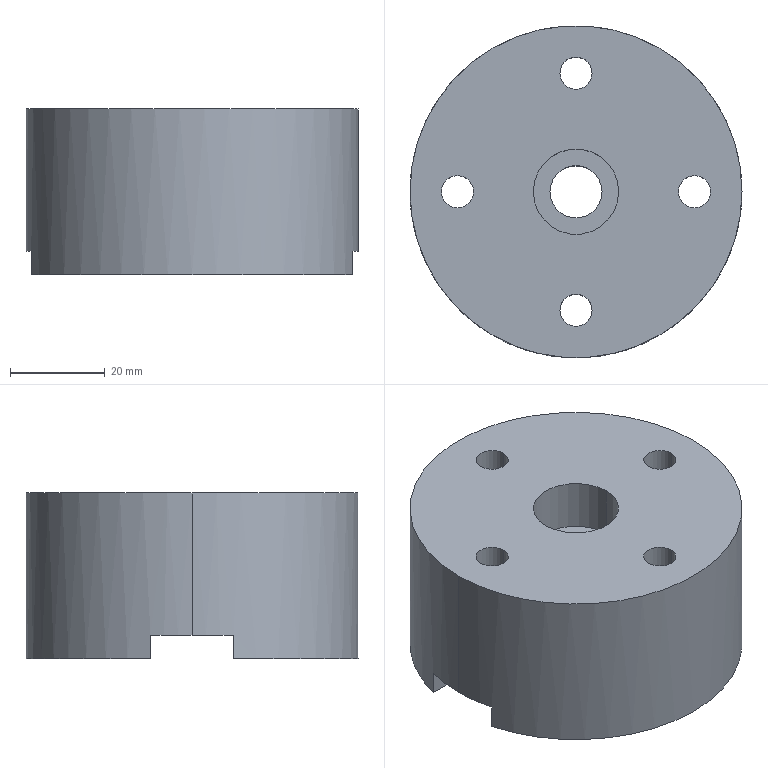Part | SolidWorks | features BaseBody 1 | 1 solid | 21 faces | box 70 x 70 x 35 mm | volume 119309 mm3 | cylinder 14 | plane 7 | commonest cylinder face diameters 6.8 x8 11 x2 18 x2 70 x2
STEP:
#1=CARTESIAN_POINT('',(-3.4,25.,35.));
#2=VERTEX_POINT('',#1);
#3=CARTESIAN_POINT('',(3.4,25.,35.));
#4=VERTEX_POINT('',#3);
#5=CARTESIAN_POINT('',(0.,25.,35.));
#6=DIRECTION('',(0.,0.,1.));
#7=DIRECTION('',(1.,0.,0.));
#8=AXIS2_PLACEMENT_3D('',#5,#6,#7);
#9=CIRCLE('',#8,3.4);
#10=EDGE_CURVE('',#2,#4,#9,.T.);
#11=ORIENTED_EDGE('',*,*,#10,.T.);
#12=CARTESIAN_POINT('',(3.4,25.,0.));
#13=VERTEX_POINT('',#12);
#14=CARTESIAN_POINT('',(3.4,25.,0.));
#15=DIRECTION('',(0.,0.,-1.));
#16=VECTOR('',#15,1000.);
#17=LINE('',#14,#16);
#18=EDGE_CURVE('',#4,#13,#17,.T.);
#19=ORIENTED_EDGE('',*,*,#18,.T.);
#20=CARTESIAN_POINT('',(-3.4,25.,0.));
#21=VERTEX_POINT('',#20);
#22=CARTESIAN_POINT('',(0.,25.,0.));
#23=DIRECTION('',(0.,0.,-1.));
#24=DIRECTION('',(-1.,0.,0.));
#25=AXIS2_PLACEMENT_3D('',#22,#23,#24);
#26=CIRCLE('',#25,3.4);
#27=EDGE_CURVE('',#13,#21,#26,.T.);
#28=ORIENTED_EDGE('',*,*,#27,.T.);
#29=CARTESIAN_POINT('',(-3.4,25.,0.));
#30=DIRECTION('',(0.,0.,-1.));
#31=VECTOR('',#30,1000.);
#32=LINE('',#29,#31);
#33=EDGE_CURVE('',#2,#21,#32,.T.);
#34=ORIENTED_EDGE('',*,*,#33,.F.);
#35=EDGE_LOOP('',(#11,#19,#28,#34));
#36=FACE_OUTER_BOUND('',#35,.T.);
#37=CARTESIAN_POINT('',(0.,25.,0.));
#38=DIRECTION('',(0.,0.,-1.));
#39=DIRECTION('',(-1.,0.,0.));
#40=AXIS2_PLACEMENT_3D('',#37,#38,#39);
#41=CYLINDRICAL_SURFACE('',#40,3.4);
#42=ADVANCED_FACE('',(#36),#41,.F.);
#43=CARTESIAN_POINT('',(21.6,0.,35.));
#44=VERTEX_POINT('',#43);
#45=CARTESIAN_POINT('',(28.4,0.,35.));
#46=VERTEX_POINT('',#45);
#47=CARTESIAN_POINT('',(25.,0.,35.));
#48=DIRECTION('',(0.,0.,1.));
#49=DIRECTION('',(1.,0.,0.));
#50=AXIS2_PLACEMENT_3D('',#47,#48,#49);
#51=CIRCLE('',#50,3.4);
#52=EDGE_CURVE('',#44,#46,#51,.T.);
#53=ORIENTED_EDGE('',*,*,#52,.T.);
#54=CARTESIAN_POINT('',(28.4,0.,5.));
#55=VERTEX_POINT('',#54);
#56=CARTESIAN_POINT('',(28.4,0.,0.));
#57=DIRECTION('',(0.,0.,-1.));
#58=VECTOR('',#57,1000.);
#59=LINE('',#56,#58);
#60=EDGE_CURVE('',#46,#55,#59,.T.);
#61=ORIENTED_EDGE('',*,*,#60,.T.);
#62=CARTESIAN_POINT('',(21.6,0.,5.));
#63=VERTEX_POINT('',#62);
#64=CARTESIAN_POINT('',(25.,0.,5.));
#65=DIRECTION('',(0.,0.,1.));
#66=DIRECTION('',(1.,0.,0.));
#67=AXIS2_PLACEMENT_3D('',#64,#65,#66);
#68=CIRCLE('',#67,3.4);
#69=EDGE_CURVE('',#63,#55,#68,.T.);
#70=ORIENTED_EDGE('',*,*,#69,.F.);
#71=CARTESIAN_POINT('',(21.6,0.,0.));
#72=DIRECTION('',(0.,0.,-1.));
#73=VECTOR('',#72,1000.);
#74=LINE('',#71,#73);
#75=EDGE_CURVE('',#44,#63,#74,.T.);
#76=ORIENTED_EDGE('',*,*,#75,.F.);
#77=EDGE_LOOP('',(#53,#61,#70,#76));
#78=FACE_OUTER_BOUND('',#77,.T.);
#79=CARTESIAN_POINT('',(25.,0.,0.));
#80=DIRECTION('',(0.,0.,-1.));
#81=DIRECTION('',(-1.,0.,0.));
#82=AXIS2_PLACEMENT_3D('',#79,#80,#81);
#83=CYLINDRICAL_SURFACE('',#82,3.4);
#84=ADVANCED_FACE('',(#78),#83,.F.);
#85=CARTESIAN_POINT('',(-28.4,0.,35.));
#86=VERTEX_POINT('',#85);
#87=CARTESIAN_POINT('',(-21.6,0.,35.));
#88=VERTEX_POINT('',#87);
#89=CARTESIAN_POINT('',(-25.,0.,35.));
#90=DIRECTION('',(0.,0.,1.));
#91=DIRECTION('',(1.,0.,0.));
#92=AXIS2_PLACEMENT_3D('',#89,#90,#91);
#93=CIRCLE('',#92,3.4);
#94=EDGE_CURVE('',#86,#88,#93,.T.);
#95=ORIENTED_EDGE('',*,*,#94,.T.);
#96=CARTESIAN_POINT('',(-21.6,0.,5.));
#97=VERTEX_POINT('',#96);
#98=CARTESIAN_POINT('',(-21.6,0.,0.));
#99=DIRECTION('',(0.,0.,-1.));
#100=VECTOR('',#99,1000.);
#101=LINE('',#98,#100);
#102=EDGE_CURVE('',#88,#97,#101,.T.);
#103=ORIENTED_EDGE('',*,*,#102,.T.);
#104=CARTESIAN_POINT('',(-28.4,0.,5.));
#105=VERTEX_POINT('',#104);
#106=CARTESIAN_POINT('',(-25.,0.,5.));
#107=DIRECTION('',(0.,0.,1.));
#108=DIRECTION('',(1.,0.,0.));
#109=AXIS2_PLACEMENT_3D('',#106,#107,#108);
#110=CIRCLE('',#109,3.4);
#111=EDGE_CURVE('',#105,#97,#110,.T.);
#112=ORIENTED_EDGE('',*,*,#111,.F.);
#113=CARTESIAN_POINT('',(-28.4,0.,0.));
#114=DIRECTION('',(0.,0.,-1.));
#115=VECTOR('',#114,1000.);
#116=LINE('',#113,#115);
#117=EDGE_CURVE('',#86,#105,#116,.T.);
#118=ORIENTED_EDGE('',*,*,#117,.F.);
#119=EDGE_LOOP('',(#95,#103,#112,#118));
#120=FACE_OUTER_BOUND('',#119,.T.);
#121=CARTESIAN_POINT('',(-25.,0.,0.));
#122=DIRECTION('',(0.,0.,-1.));
#123=DIRECTION('',(-1.,0.,0.));
#124=AXIS2_PLACEMENT_3D('',#121,#122,#123);
#125=CYLINDRICAL_SURFACE('',#124,3.4);
#126=ADVANCED_FACE('',(#120),#125,.F.);
#127=CARTESIAN_POINT('',(-3.4,-25.,35.));
#128=VERTEX_POINT('',#127);
#129=CARTESIAN_POINT('',(3.4,-25.,35.));
#130=VERTEX_POINT('',#129);
#131=CARTESIAN_POINT('',(0.,-25.,35.));
#132=DIRECTION('',(0.,0.,1.));
#133=DIRECTION('',(1.,0.,0.));
#134=AXIS2_PLACEMENT_3D('',#131,#132,#133);
#135=CIRCLE('',#134,3.4);
#136=EDGE_CURVE('',#128,#130,#135,.T.);
#137=ORIENTED_EDGE('',*,*,#136,.T.);
#138=CARTESIAN_POINT('',(3.4,-25.,0.));
#139=VERTEX_POINT('',#138);
#140=CARTESIAN_POINT('',(3.4,-25.,0.));
#141=DIRECTION('',(0.,0.,-1.));
#142=VECTOR('',#141,1000.);
#143=LINE('',#140,#142);
#144=EDGE_CURVE('',#130,#139,#143,.T.);
#145=ORIENTED_EDGE('',*,*,#144,.T.);
#146=CARTESIAN_POINT('',(-3.4,-25.,0.));
#147=VERTEX_POINT('',#146);
#148=CARTESIAN_POINT('',(0.,-25.,0.));
#149=DIRECTION('',(0.,0.,-1.));
#150=DIRECTION('',(-1.,0.,0.));
#151=AXIS2_PLACEMENT_3D('',#148,#149,#150);
#152=CIRCLE('',#151,3.4);
#153=EDGE_CURVE('',#139,#147,#152,.T.);
#154=ORIENTED_EDGE('',*,*,#153,.T.);
#155=CARTESIAN_POINT('',(-3.4,-25.,0.));
#156=DIRECTION('',(0.,0.,-1.));
#157=VECTOR('',#156,1000.);
#158=LINE('',#155,#157);
#159=EDGE_CURVE('',#128,#147,#158,.T.);
#160=ORIENTED_EDGE('',*,*,#159,.F.);
#161=EDGE_LOOP('',(#137,#145,#154,#160));
#162=FACE_OUTER_BOUND('',#161,.T.);
#163=CARTESIAN_POINT('',(0.,-25.,0.));
#164=DIRECTION('',(0.,0.,-1.));
#165=DIRECTION('',(-1.,0.,0.));
#166=AXIS2_PLACEMENT_3D('',#163,#164,#165);
#167=CYLINDRICAL_SURFACE('',#166,3.4);
#168=ADVANCED_FACE('',(#162),#167,.F.);
#169=CARTESIAN_POINT('',(-9.,0.,24.));
#170=VERTEX_POINT('',#169);
#171=CARTESIAN_POINT('',(9.,0.,24.));
#172=VERTEX_POINT('',#171);
#173=CARTESIAN_POINT('',(0.,0.,24.));
#174=DIRECTION('',(0.,0.,1.));
#175=DIRECTION('',(1.,0.,0.));
#176=AXIS2_PLACEMENT_3D('',#173,#174,#175);
#177=CIRCLE('',#176,9.);
#178=EDGE_CURVE('',#170,#172,#177,.T.);
#179=ORIENTED_EDGE('',*,*,#178,.F.);
#180=CARTESIAN_POINT('',(-9.,0.,35.));
#181=VERTEX_POINT('',#180);
#182=CARTESIAN_POINT('',(-9.,0.,35.));
#183=DIRECTION('',(0.,0.,1.));
#184=VECTOR('',#183,1000.);
#185=LINE('',#182,#184);
#186=EDGE_CURVE('',#170,#181,#185,.T.);
#187=ORIENTED_EDGE('',*,*,#186,.T.);
#188=CARTESIAN_POINT('',(9.,0.,35.));
#189=VERTEX_POINT('',#188);
#190=CARTESIAN_POINT('',(0.,0.,35.));
#191=DIRECTION('',(0.,0.,1.));
#192=DIRECTION('',(1.,0.,0.));
#193=AXIS2_PLACEMENT_3D('',#190,#191,#192);
#194=CIRCLE('',#193,9.);
#195=EDGE_CURVE('',#181,#189,#194,.T.);
#196=ORIENTED_EDGE('',*,*,#195,.T.);
#197=CARTESIAN_POINT('',(9.,0.,35.));
#198=DIRECTION('',(0.,0.,1.));
#199=VECTOR('',#198,1000.);
#200=LINE('',#197,#199);
#201=EDGE_CURVE('',#172,#189,#200,.T.);
#202=ORIENTED_EDGE('',*,*,#201,.F.);
#203=EDGE_LOOP('',(#179,#187,#196,#202));
#204=FACE_OUTER_BOUND('',#203,.T.);
#205=CARTESIAN_POINT('',(0.,0.,35.));
#206=DIRECTION('',(0.,0.,1.));
#207=DIRECTION('',(1.,0.,0.));
#208=AXIS2_PLACEMENT_3D('',#205,#206,#207);
#209=CYLINDRICAL_SURFACE('',#208,9.);
#210=ADVANCED_FACE('',(#204),#209,.F.);
#211=CARTESIAN_POINT('',(-5.5,0.,5.));
#212=VERTEX_POINT('',#211);
#213=CARTESIAN_POINT('',(5.5,0.,5.));
#214=VERTEX_POINT('',#213);
#215=CARTESIAN_POINT('',(0.,0.,5.));
#216=DIRECTION('',(0.,0.,1.));
#217=DIRECTION('',(1.,0.,0.));
#218=AXIS2_PLACEMENT_3D('',#215,#216,#217);
#219=CIRCLE('',#218,5.5);
#220=EDGE_CURVE('',#212,#214,#219,.T.);
#221=ORIENTED_EDGE('',*,*,#220,.F.);
#222=CARTESIAN_POINT('',(-5.5,0.,24.));
#223=VERTEX_POINT('',#222);
#224=CARTESIAN_POINT('',(-5.5,0.,35.));
#225=DIRECTION('',(0.,0.,1.));
#226=VECTOR('',#225,1000.);
#227=LINE('',#224,#226);
#228=EDGE_CURVE('',#212,#223,#227,.T.);
#229=ORIENTED_EDGE('',*,*,#228,.T.);
#230=CARTESIAN_POINT('',(5.5,0.,24.));
#231=VERTEX_POINT('',#230);
#232=CARTESIAN_POINT('',(0.,0.,24.));
#233=DIRECTION('',(0.,0.,1.));
#234=DIRECTION('',(1.,0.,0.));
#235=AXIS2_PLACEMENT_3D('',#232,#233,#234);
#236=CIRCLE('',#235,5.5);
#237=EDGE_CURVE('',#223,#231,#236,.T.);
#238=ORIENTED_EDGE('',*,*,#237,.T.);
#239=CARTESIAN_POINT('',(5.5,0.,35.));
#240=DIRECTION('',(0.,0.,1.));
#241=VECTOR('',#240,1000.);
#242=LINE('',#239,#241);
#243=EDGE_CURVE('',#214,#231,#242,.T.);
#244=ORIENTED_EDGE('',*,*,#243,.F.);
#245=EDGE_LOOP('',(#221,#229,#238,#244));
#246=FACE_OUTER_BOUND('',#245,.T.);
#247=CARTESIAN_POINT('',(0.,0.,35.));
#248=DIRECTION('',(0.,0.,1.));
#249=DIRECTION('',(1.,0.,0.));
#250=AXIS2_PLACEMENT_3D('',#247,#248,#249);
#251=CYLINDRICAL_SURFACE('',#250,5.5);
#252=ADVANCED_FACE('',(#246),#251,.F.);
#253=CARTESIAN_POINT('',(35.,0.,35.));
#254=VERTEX_POINT('',#253);
#255=CARTESIAN_POINT('',(-35.,0.,35.));
#256=VERTEX_POINT('',#255);
#257=CARTESIAN_POINT('',(0.,0.,35.));
#258=DIRECTION('',(0.,0.,1.));
#259=DIRECTION('',(1.,0.,0.));
#260=AXIS2_PLACEMENT_3D('',#257,#258,#259);
#261=CIRCLE('',#260,35.);
#262=EDGE_CURVE('',#254,#256,#261,.T.);
#263=ORIENTED_EDGE('',*,*,#262,.F.);
#264=CARTESIAN_POINT('',(35.,0.,5.));
#265=VERTEX_POINT('',#264);
#266=CARTESIAN_POINT('',(35.,0.,35.));
#267=DIRECTION('',(0.,0.,-1.));
#268=VECTOR('',#267,1000.);
#269=LINE('',#266,#268);
#270=EDGE_CURVE('',#254,#265,#269,.T.);
#271=ORIENTED_EDGE('',*,*,#270,.T.);
#272=CARTESIAN_POINT('',(33.889,8.75,5.));
#273=VERTEX_POINT('',#272);
#274=CARTESIAN_POINT('',(0.,0.,5.));
#275=DIRECTION('',(0.,0.,1.));
#276=DIRECTION('',(1.,0.,0.));
#277=AXIS2_PLACEMENT_3D('',#274,#275,#276);
#278=CIRCLE('',#277,35.);
#279=EDGE_CURVE('',#265,#273,#278,.T.);
#280=ORIENTED_EDGE('',*,*,#279,.T.);
#281=CARTESIAN_POINT('',(33.889,8.75,0.));
#282=VERTEX_POINT('',#281);
#283=CARTESIAN_POINT('',(33.889,8.75,35.));
#284=DIRECTION('',(0.,0.,-1.));
#285=VECTOR('',#284,1000.);
#286=LINE('',#283,#285);
#287=EDGE_CURVE('',#273,#282,#286,.T.);
#288=ORIENTED_EDGE('',*,*,#287,.T.);
#289=CARTESIAN_POINT('',(-33.889,8.75,0.));
#290=VERTEX_POINT('',#289);
#291=CARTESIAN_POINT('',(0.,0.,0.));
#292=DIRECTION('',(0.,0.,1.));
#293=DIRECTION('',(1.,0.,0.));
#294=AXIS2_PLACEMENT_3D('',#291,#292,#293);
#295=CIRCLE('',#294,35.);
#296=EDGE_CURVE('',#282,#290,#295,.T.);
#297=ORIENTED_EDGE('',*,*,#296,.T.);
#298=CARTESIAN_POINT('',(-33.889,8.75,5.));
#299=VERTEX_POINT('',#298);
#300=CARTESIAN_POINT('',(-33.889,8.75,35.));
#301=DIRECTION('',(0.,0.,1.));
#302=VECTOR('',#301,1000.);
#303=LINE('',#300,#302);
#304=EDGE_CURVE('',#290,#299,#303,.T.);
#305=ORIENTED_EDGE('',*,*,#304,.T.);
#306=CARTESIAN_POINT('',(-35.,0.,5.));
#307=VERTEX_POINT('',#306);
#308=CARTESIAN_POINT('',(0.,0.,5.));
#309=DIRECTION('',(0.,0.,1.));
#310=DIRECTION('',(1.,0.,0.));
#311=AXIS2_PLACEMENT_3D('',#308,#309,#310);
#312=CIRCLE('',#311,35.);
#313=EDGE_CURVE('',#299,#307,#312,.T.);
#314=ORIENTED_EDGE('',*,*,#313,.T.);
#315=CARTESIAN_POINT('',(-35.,0.,35.));
#316=DIRECTION('',(0.,0.,-1.));
#317=VECTOR('',#316,1000.);
#318=LINE('',#315,#317);
#319=EDGE_CURVE('',#256,#307,#318,.T.);
#320=ORIENTED_EDGE('',*,*,#319,.F.);
#321=EDGE_LOOP('',(#263,#271,#280,#288,#297,#305,#314,#320));
#322=FACE_OUTER_BOUND('',#321,.T.);
#323=CARTESIAN_POINT('',(0.,0.,35.));
#324=DIRECTION('',(0.,0.,-1.));
#325=DIRECTION('',(-1.,0.,0.));
#326=AXIS2_PLACEMENT_3D('',#323,#324,#325);
#327=CYLINDRICAL_SURFACE('',#326,35.);
#328=ADVANCED_FACE('',(#322),#327,.T.);
#329=CARTESIAN_POINT('',(0.,25.,0.));
#330=DIRECTION('',(0.,0.,-1.));
#331=DIRECTION('',(-1.,0.,0.));
#332=AXIS2_PLACEMENT_3D('',#329,#330,#331);
#333=CIRCLE('',#332,3.4);
#334=EDGE_CURVE('',#21,#13,#333,.T.);
#335=ORIENTED_EDGE('',*,*,#334,.F.);
#336=ORIENTED_EDGE('',*,*,#27,.F.);
#337=EDGE_LOOP('',(#335,#336));
#338=FACE_BOUND('',#337,.T.);
#339=ORIENTED_EDGE('',*,*,#296,.F.);
#340=CARTESIAN_POINT('',(0.,8.75,0.));
#341=DIRECTION('',(-1.,0.,0.));
#342=VECTOR('',#341,1000.);
#343=LINE('',#340,#342);
#344=EDGE_CURVE('',#282,#290,#343,.T.);
#345=ORIENTED_EDGE('',*,*,#344,.T.);
#346=EDGE_LOOP('',(#339,#345));
#347=FACE_OUTER_BOUND('',#346,.T.);
#348=CARTESIAN_POINT('',(0.,0.,0.));
#349=DIRECTION('',(0.,0.,1.));
#350=DIRECTION('',(1.,0.,0.));
#351=AXIS2_PLACEMENT_3D('',#348,#349,#350);
#352=PLANE('',#351);
#353=ADVANCED_FACE('',(#338,#347),#352,.F.);
#354=ORIENTED_EDGE('',*,*,#270,.F.);
#355=CARTESIAN_POINT('',(0.,0.,35.));
#356=DIRECTION('',(0.,0.,1.));
#357=DIRECTION('',(1.,0.,0.));
#358=AXIS2_PLACEMENT_3D('',#355,#356,#357);
#359=CIRCLE('',#358,35.);
#360=EDGE_CURVE('',#256,#254,#359,.T.);
#361=ORIENTED_EDGE('',*,*,#360,.F.);
#362=ORIENTED_EDGE('',*,*,#319,.T.);
#363=CARTESIAN_POINT('',(-33.889,-8.75,5.));
#364=VERTEX_POINT('',#363);
#365=CARTESIAN_POINT('',(0.,0.,5.));
#366=DIRECTION('',(0.,0.,1.));
#367=DIRECTION('',(1.,0.,0.));
#368=AXIS2_PLACEMENT_3D('',#365,#366,#367);
#369=CIRCLE('',#368,35.);
#370=EDGE_CURVE('',#307,#364,#369,.T.);
#371=ORIENTED_EDGE('',*,*,#370,.T.);
#372=CARTESIAN_POINT('',(-33.889,-8.75,0.));
#373=VERTEX_POINT('',#372);
#374=CARTESIAN_POINT('',(-33.889,-8.75,35.));
#375=DIRECTION('',(0.,0.,-1.));
#376=VECTOR('',#375,1000.);
#377=LINE('',#374,#376);
#378=EDGE_CURVE('',#364,#373,#377,.T.);
#379=ORIENTED_EDGE('',*,*,#378,.T.);
#380=CARTESIAN_POINT('',(33.889,-8.75,0.));
#381=VERTEX_POINT('',#380);
#382=CARTESIAN_POINT('',(0.,0.,0.));
#383=DIRECTION('',(0.,0.,1.));
#384=DIRECTION('',(1.,0.,0.));
#385=AXIS2_PLACEMENT_3D('',#382,#383,#384);
#386=CIRCLE('',#385,35.);
#387=EDGE_CURVE('',#373,#381,#386,.T.);
#388=ORIENTED_EDGE('',*,*,#387,.T.);
#389=CARTESIAN_POINT('',(33.889,-8.75,5.));
#390=VERTEX_POINT('',#389);
#391=CARTESIAN_POINT('',(33.889,-8.75,35.));
#392=DIRECTION('',(0.,0.,1.));
#393=VECTOR('',#392,1000.);
#394=LINE('',#391,#393);
#395=EDGE_CURVE('',#381,#390,#394,.T.);
#396=ORIENTED_EDGE('',*,*,#395,.T.);
#397=CARTESIAN_POINT('',(0.,0.,5.));
#398=DIRECTION('',(0.,0.,1.));
#399=DIRECTION('',(1.,0.,0.));
#400=AXIS2_PLACEMENT_3D('',#397,#398,#399);
#401=CIRCLE('',#400,35.);
#402=EDGE_CURVE('',#390,#265,#401,.T.);
#403=ORIENTED_EDGE('',*,*,#402,.T.);
#404=EDGE_LOOP('',(#354,#361,#362,#371,#379,#388,#396,#403));
#405=FACE_OUTER_BOUND('',#404,.T.);
#406=CARTESIAN_POINT('',(0.,0.,35.));
#407=DIRECTION('',(0.,0.,-1.));
#408=DIRECTION('',(-1.,0.,0.));
#409=AXIS2_PLACEMENT_3D('',#406,#407,#408);
#410=CYLINDRICAL_SURFACE('',#409,35.);
#411=ADVANCED_FACE('',(#405),#410,.T.);
#412=ORIENTED_EDGE('',*,*,#10,.F.);
#413=CARTESIAN_POINT('',(0.,25.,35.));
#414=DIRECTION('',(0.,0.,1.));
#415=DIRECTION('',(1.,0.,0.));
#416=AXIS2_PLACEMENT_3D('',#413,#414,#415);
#417=CIRCLE('',#416,3.4);
#418=EDGE_CURVE('',#4,#2,#417,.T.);
#419=ORIENTED_EDGE('',*,*,#418,.F.);
#420=EDGE_LOOP('',(#412,#419));
#421=FACE_BOUND('',#420,.T.);
#422=ORIENTED_EDGE('',*,*,#52,.F.);
#423=CARTESIAN_POINT('',(25.,0.,35.));
#424=DIRECTION('',(0.,0.,1.));
#425=DIRECTION('',(1.,0.,0.));
#426=AXIS2_PLACEMENT_3D('',#423,#424,#425);
#427=CIRCLE('',#426,3.4);
#428=EDGE_CURVE('',#46,#44,#427,.T.);
#429=ORIENTED_EDGE('',*,*,#428,.F.);
#430=EDGE_LOOP('',(#422,#429));
#431=FACE_BOUND('',#430,.T.);
#432=ORIENTED_EDGE('',*,*,#94,.F.);
#433=CARTESIAN_POINT('',(-25.,0.,35.));
#434=DIRECTION('',(0.,0.,1.));
#435=DIRECTION('',(1.,0.,0.));
#436=AXIS2_PLACEMENT_3D('',#433,#434,#435);
#437=CIRCLE('',#436,3.4);
#438=EDGE_CURVE('',#88,#86,#437,.T.);
#439=ORIENTED_EDGE('',*,*,#438,.F.);
#440=EDGE_LOOP('',(#432,#439));
#441=FACE_BOUND('',#440,.T.);
#442=ORIENTED_EDGE('',*,*,#136,.F.);
#443=CARTESIAN_POINT('',(0.,-25.,35.));
#444=DIRECTION('',(0.,0.,1.));
#445=DIRECTION('',(1.,0.,0.));
#446=AXIS2_PLACEMENT_3D('',#443,#444,#445);
#447=CIRCLE('',#446,3.4);
#448=EDGE_CURVE('',#130,#128,#447,.T.);
#449=ORIENTED_EDGE('',*,*,#448,.F.);
#450=EDGE_LOOP('',(#442,#449));
#451=FACE_BOUND('',#450,.T.);
#452=CARTESIAN_POINT('',(0.,0.,35.));
#453=DIRECTION('',(0.,0.,1.));
#454=DIRECTION('',(1.,0.,0.));
#455=AXIS2_PLACEMENT_3D('',#452,#453,#454);
#456=CIRCLE('',#455,9.);
#457=EDGE_CURVE('',#189,#181,#456,.T.);
#458=ORIENTED_EDGE('',*,*,#457,.F.);
#459=ORIENTED_EDGE('',*,*,#195,.F.);
#460=EDGE_LOOP('',(#458,#459));
#461=FACE_BOUND('',#460,.T.);
#462=ORIENTED_EDGE('',*,*,#360,.T.);
#463=ORIENTED_EDGE('',*,*,#262,.T.);
#464=EDGE_LOOP('',(#462,#463));
#465=FACE_OUTER_BOUND('',#464,.T.);
#466=CARTESIAN_POINT('',(0.,0.,35.));
#467=DIRECTION('',(0.,0.,1.));
#468=DIRECTION('',(1.,0.,0.));
#469=AXIS2_PLACEMENT_3D('',#466,#467,#468);
#470=PLANE('',#469);
#471=ADVANCED_FACE('',(#421,#431,#441,#451,#461,#465),#470,.T.);
#472=CARTESIAN_POINT('',(0.,-25.,0.));
#473=DIRECTION('',(0.,0.,-1.));
#474=DIRECTION('',(-1.,0.,0.));
#475=AXIS2_PLACEMENT_3D('',#472,#473,#474);
#476=CIRCLE('',#475,3.4);
#477=EDGE_CURVE('',#147,#139,#476,.T.);
#478=ORIENTED_EDGE('',*,*,#477,.F.);
#479=ORIENTED_EDGE('',*,*,#153,.F.);
#480=EDGE_LOOP('',(#478,#479));
#481=FACE_BOUND('',#480,.T.);
#482=ORIENTED_EDGE('',*,*,#387,.F.);
#483=CARTESIAN_POINT('',(0.,-8.75,0.));
#484=DIRECTION('',(1.,0.,0.));
#485=VECTOR('',#484,1000.);
#486=LINE('',#483,#485);
#487=EDGE_CURVE('',#373,#381,#486,.T.);
#488=ORIENTED_EDGE('',*,*,#487,.T.);
#489=EDGE_LOOP('',(#482,#488));
#490=FACE_OUTER_BOUND('',#489,.T.);
#491=CARTESIAN_POINT('',(0.,0.,0.));
#492=DIRECTION('',(0.,0.,1.));
#493=DIRECTION('',(1.,0.,0.));
#494=AXIS2_PLACEMENT_3D('',#491,#492,#493);
#495=PLANE('',#494);
#496=ADVANCED_FACE('',(#481,#490),#495,.F.);
#497=ORIENTED_EDGE('',*,*,#69,.T.);
#498=CARTESIAN_POINT('',(25.,0.,5.));
#499=DIRECTION('',(0.,0.,1.));
#500=DIRECTION('',(1.,0.,0.));
#501=AXIS2_PLACEMENT_3D('',#498,#499,#500);
#502=CIRCLE('',#501,3.4);
#503=EDGE_CURVE('',#55,#63,#502,.T.);
#504=ORIENTED_EDGE('',*,*,#503,.T.);
#505=EDGE_LOOP('',(#497,#504));
#506=FACE_BOUND('',#505,.T.);
#507=ORIENTED_EDGE('',*,*,#111,.T.);
#508=CARTESIAN_POINT('',(-25.,0.,5.));
#509=DIRECTION('',(0.,0.,1.));
#510=DIRECTION('',(1.,0.,0.));
#511=AXIS2_PLACEMENT_3D('',#508,#509,#510);
#512=CIRCLE('',#511,3.4);
#513=EDGE_CURVE('',#97,#105,#512,.T.);
#514=ORIENTED_EDGE('',*,*,#513,.T.);
#515=EDGE_LOOP('',(#507,#514));
#516=FACE_BOUND('',#515,.T.);
#517=CARTESIAN_POINT('',(0.,0.,5.));
#518=DIRECTION('',(0.,0.,1.));
#519=DIRECTION('',(1.,0.,0.));
#520=AXIS2_PLACEMENT_3D('',#517,#518,#519);
#521=CIRCLE('',#520,5.5);
#522=EDGE_CURVE('',#214,#212,#521,.T.);
#523=ORIENTED_EDGE('',*,*,#522,.T.);
#524=ORIENTED_EDGE('',*,*,#220,.T.);
#525=EDGE_LOOP('',(#523,#524));
#526=FACE_BOUND('',#525,.T.);
#527=CARTESIAN_POINT('',(-114.,8.75,5.));
#528=DIRECTION('',(1.,0.,0.));
#529=VECTOR('',#528,1000.);
#530=LINE('',#527,#529);
#531=EDGE_CURVE('',#299,#273,#530,.T.);
#532=ORIENTED_EDGE('',*,*,#531,.T.);
#533=ORIENTED_EDGE('',*,*,#279,.F.);
#534=ORIENTED_EDGE('',*,*,#402,.F.);
#535=CARTESIAN_POINT('',(-114.,-8.75,5.));
#536=DIRECTION('',(1.,0.,0.));
#537=VECTOR('',#536,1000.);
#538=LINE('',#535,#537);
#539=EDGE_CURVE('',#364,#390,#538,.T.);
#540=ORIENTED_EDGE('',*,*,#539,.F.);
#541=ORIENTED_EDGE('',*,*,#370,.F.);
#542=ORIENTED_EDGE('',*,*,#313,.F.);
#543=EDGE_LOOP('',(#532,#533,#534,#540,#541,#542));
#544=FACE_OUTER_BOUND('',#543,.T.);
#545=CARTESIAN_POINT('',(-114.,-8.75,5.));
#546=DIRECTION('',(0.,0.,1.));
#547=DIRECTION('',(1.,0.,0.));
#548=AXIS2_PLACEMENT_3D('',#545,#546,#547);
#549=PLANE('',#548);
#550=ADVANCED_FACE('',(#506,#516,#526,#544),#549,.F.);
#551=ORIENTED_EDGE('',*,*,#531,.F.);
#552=ORIENTED_EDGE('',*,*,#304,.F.);
#553=ORIENTED_EDGE('',*,*,#344,.F.);
#554=ORIENTED_EDGE('',*,*,#287,.F.);
#555=EDGE_LOOP('',(#551,#552,#553,#554));
#556=FACE_OUTER_BOUND('',#555,.T.);
#557=CARTESIAN_POINT('',(-114.,8.75,5.));
#558=DIRECTION('',(0.,1.,0.));
#559=DIRECTION('',(0.,0.,1.));
#560=AXIS2_PLACEMENT_3D('',#557,#558,#559);
#561=PLANE('',#560);
#562=ADVANCED_FACE('',(#556),#561,.F.);
#563=ORIENTED_EDGE('',*,*,#539,.T.);
#564=ORIENTED_EDGE('',*,*,#395,.F.);
#565=ORIENTED_EDGE('',*,*,#487,.F.);
#566=ORIENTED_EDGE('',*,*,#378,.F.);
#567=EDGE_LOOP('',(#563,#564,#565,#566));
#568=FACE_OUTER_BOUND('',#567,.T.);
#569=CARTESIAN_POINT('',(-114.,-8.75,5.));
#570=DIRECTION('',(0.,-1.,0.));
#571=DIRECTION('',(0.,0.,-1.));
#572=AXIS2_PLACEMENT_3D('',#569,#570,#571);
#573=PLANE('',#572);
#574=ADVANCED_FACE('',(#568),#573,.F.);
#575=ORIENTED_EDGE('',*,*,#228,.F.);
#576=ORIENTED_EDGE('',*,*,#522,.F.);
#577=ORIENTED_EDGE('',*,*,#243,.T.);
#578=CARTESIAN_POINT('',(0.,0.,24.));
#579=DIRECTION('',(0.,0.,1.));
#580=DIRECTION('',(1.,0.,0.));
#581=AXIS2_PLACEMENT_3D('',#578,#579,#580);
#582=CIRCLE('',#581,5.5);
#583=EDGE_CURVE('',#231,#223,#582,.T.);
#584=ORIENTED_EDGE('',*,*,#583,.T.);
#585=EDGE_LOOP('',(#575,#576,#577,#584));
#586=FACE_OUTER_BOUND('',#585,.T.);
#587=CARTESIAN_POINT('',(0.,0.,35.));
#588=DIRECTION('',(0.,0.,1.));
#589=DIRECTION('',(1.,0.,0.));
#590=AXIS2_PLACEMENT_3D('',#587,#588,#589);
#591=CYLINDRICAL_SURFACE('',#590,5.5);
#592=ADVANCED_FACE('',(#586),#591,.F.);
#593=ORIENTED_EDGE('',*,*,#583,.F.);
#594=ORIENTED_EDGE('',*,*,#237,.F.);
#595=EDGE_LOOP('',(#593,#594));
#596=FACE_BOUND('',#595,.T.);
#597=CARTESIAN_POINT('',(0.,0.,24.));
#598=DIRECTION('',(0.,0.,1.));
#599=DIRECTION('',(1.,0.,0.));
#600=AXIS2_PLACEMENT_3D('',#597,#598,#599);
#601=CIRCLE('',#600,9.);
#602=EDGE_CURVE('',#172,#170,#601,.T.);
#603=ORIENTED_EDGE('',*,*,#602,.T.);
#604=ORIENTED_EDGE('',*,*,#178,.T.);
#605=EDGE_LOOP('',(#603,#604));
#606=FACE_OUTER_BOUND('',#605,.T.);
#607=CARTESIAN_POINT('',(5.5,0.,24.));
#608=DIRECTION('',(0.,0.,-1.));
#609=DIRECTION('',(-1.,0.,0.));
#610=AXIS2_PLACEMENT_3D('',#607,#608,#609);
#611=PLANE('',#610);
#612=ADVANCED_FACE('',(#596,#606),#611,.F.);
#613=ORIENTED_EDGE('',*,*,#186,.F.);
#614=ORIENTED_EDGE('',*,*,#602,.F.);
#615=ORIENTED_EDGE('',*,*,#201,.T.);
#616=ORIENTED_EDGE('',*,*,#457,.T.);
#617=EDGE_LOOP('',(#613,#614,#615,#616));
#618=FACE_OUTER_BOUND('',#617,.T.);
#619=CARTESIAN_POINT('',(0.,0.,35.));
#620=DIRECTION('',(0.,0.,1.));
#621=DIRECTION('',(1.,0.,0.));
#622=AXIS2_PLACEMENT_3D('',#619,#620,#621);
#623=CYLINDRICAL_SURFACE('',#622,9.);
#624=ADVANCED_FACE('',(#618),#623,.F.);
#625=ORIENTED_EDGE('',*,*,#144,.F.);
#626=ORIENTED_EDGE('',*,*,#448,.T.);
#627=ORIENTED_EDGE('',*,*,#159,.T.);
#628=ORIENTED_EDGE('',*,*,#477,.T.);
#629=EDGE_LOOP('',(#625,#626,#627,#628));
#630=FACE_OUTER_BOUND('',#629,.T.);
#631=CARTESIAN_POINT('',(0.,-25.,0.));
#632=DIRECTION('',(0.,0.,-1.));
#633=DIRECTION('',(-1.,0.,0.));
#634=AXIS2_PLACEMENT_3D('',#631,#632,#633);
#635=CYLINDRICAL_SURFACE('',#634,3.4);
#636=ADVANCED_FACE('',(#630),#635,.F.);
#637=ORIENTED_EDGE('',*,*,#102,.F.);
#638=ORIENTED_EDGE('',*,*,#438,.T.);
#639=ORIENTED_EDGE('',*,*,#117,.T.);
#640=ORIENTED_EDGE('',*,*,#513,.F.);
#641=EDGE_LOOP('',(#637,#638,#639,#640));
#642=FACE_OUTER_BOUND('',#641,.T.);
#643=CARTESIAN_POINT('',(-25.,0.,0.));
#644=DIRECTION('',(0.,0.,-1.));
#645=DIRECTION('',(-1.,0.,0.));
#646=AXIS2_PLACEMENT_3D('',#643,#644,#645);
#647=CYLINDRICAL_SURFACE('',#646,3.4);
#648=ADVANCED_FACE('',(#642),#647,.F.);
#649=ORIENTED_EDGE('',*,*,#60,.F.);
#650=ORIENTED_EDGE('',*,*,#428,.T.);
#651=ORIENTED_EDGE('',*,*,#75,.T.);
#652=ORIENTED_EDGE('',*,*,#503,.F.);
#653=EDGE_LOOP('',(#649,#650,#651,#652));
#654=FACE_OUTER_BOUND('',#653,.T.);
#655=CARTESIAN_POINT('',(25.,0.,0.));
#656=DIRECTION('',(0.,0.,-1.));
#657=DIRECTION('',(-1.,0.,0.));
#658=AXIS2_PLACEMENT_3D('',#655,#656,#657);
#659=CYLINDRICAL_SURFACE('',#658,3.4);
#660=ADVANCED_FACE('',(#654),#659,.F.);
#661=ORIENTED_EDGE('',*,*,#18,.F.);
#662=ORIENTED_EDGE('',*,*,#418,.T.);
#663=ORIENTED_EDGE('',*,*,#33,.T.);
#664=ORIENTED_EDGE('',*,*,#334,.T.);
#665=EDGE_LOOP('',(#661,#662,#663,#664));
#666=FACE_OUTER_BOUND('',#665,.T.);
#667=CARTESIAN_POINT('',(0.,25.,0.));
#668=DIRECTION('',(0.,0.,-1.));
#669=DIRECTION('',(-1.,0.,0.));
#670=AXIS2_PLACEMENT_3D('',#667,#668,#669);
#671=CYLINDRICAL_SURFACE('',#670,3.4);
#672=ADVANCED_FACE('',(#666),#671,.F.);
#673=CLOSED_SHELL('',(#42,#84,#126,#168,#210,#252,#328,#353,#411,#471,#496,#550,#562,#574,#592,#612,#624,#636,#648,#660,#672));
#674=MANIFOLD_SOLID_BREP('',#673);
#675=CARTESIAN_POINT('',(0.,0.,0.));
#676=DIRECTION('',(0.,0.,1.));
#677=DIRECTION('',(1.,0.,0.));
#678=AXIS2_PLACEMENT_3D('',#675,#676,#677);
#679=(LENGTH_UNIT()NAMED_UNIT(*)SI_UNIT(.MILLI.,.METRE.));
#680=UNCERTAINTY_MEASURE_WITH_UNIT(LENGTH_MEASURE(0.00001),#679,'','');
#681=(NAMED_UNIT(*)PLANE_ANGLE_UNIT()SI_UNIT($,.RADIAN.));
#682=(NAMED_UNIT(*)SI_UNIT($,.STERADIAN.)SOLID_ANGLE_UNIT());
#683=(GEOMETRIC_REPRESENTATION_CONTEXT(3)GLOBAL_UNCERTAINTY_ASSIGNED_CONTEXT((#680))GLOBAL_UNIT_ASSIGNED_CONTEXT((#679,#681,#682))REPRESENTATION_CONTEXT('',''));
#684=ADVANCED_BREP_SHAPE_REPRESENTATION('',(#674,#678),#683);